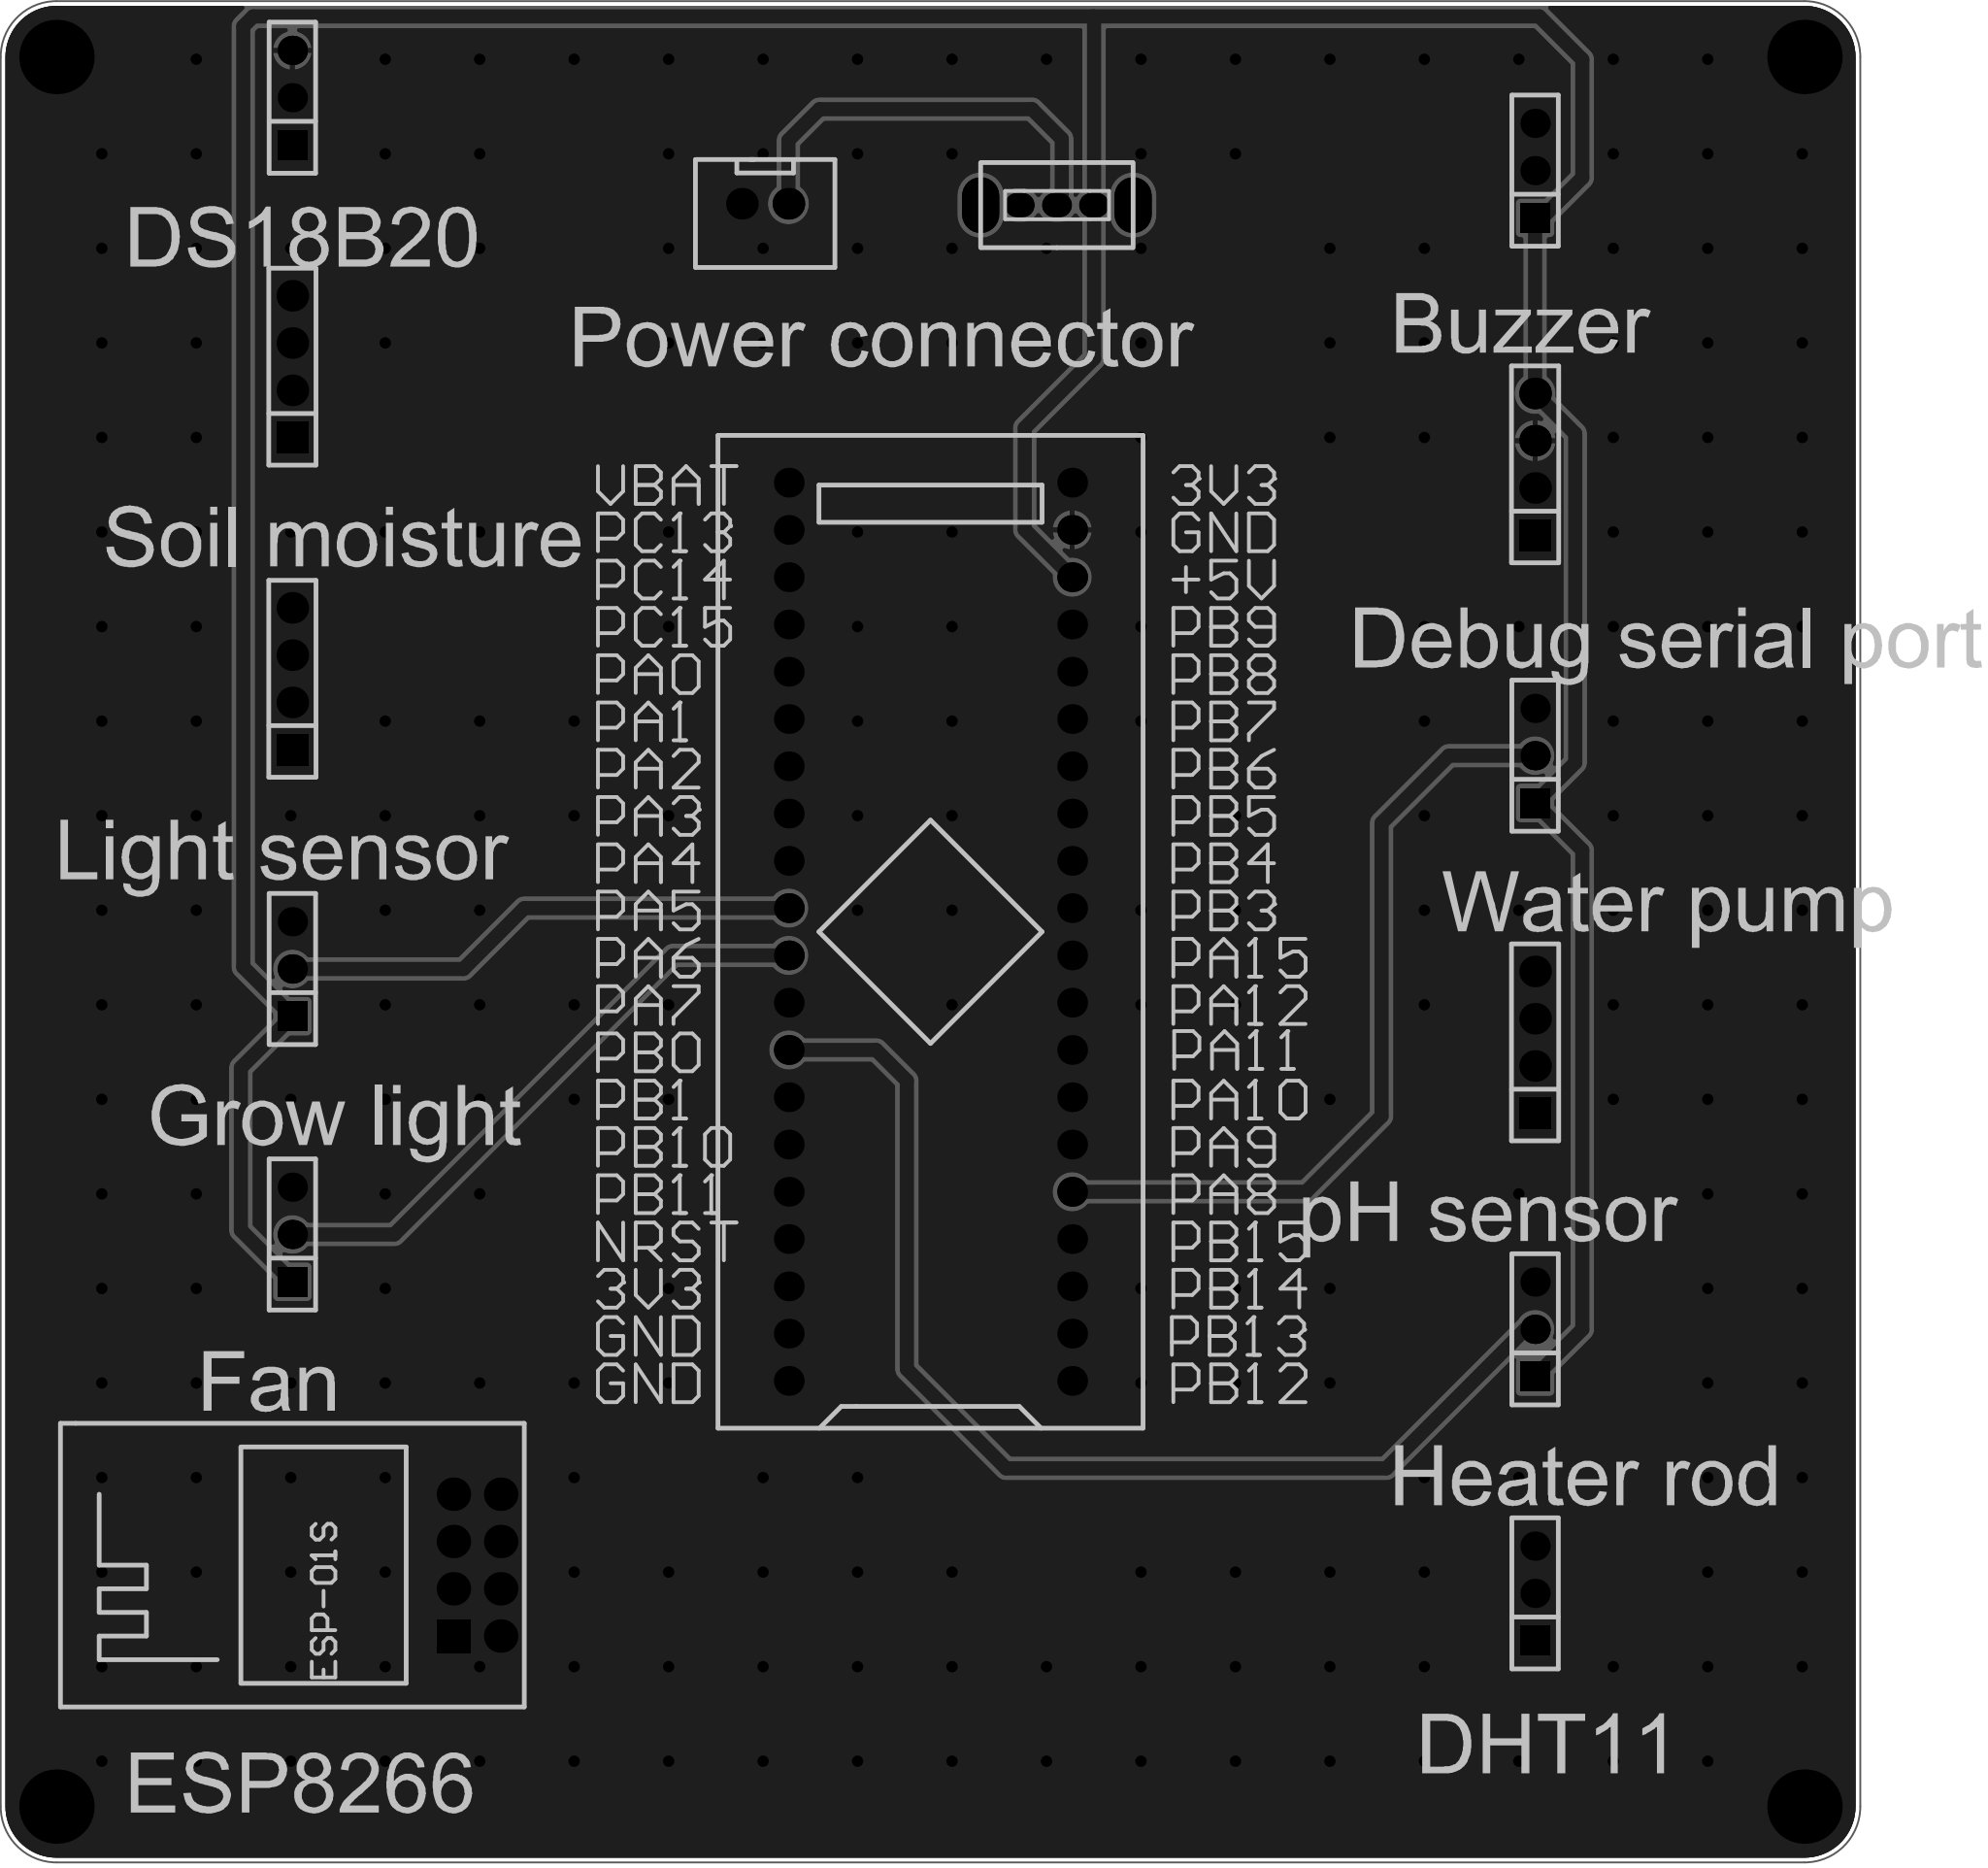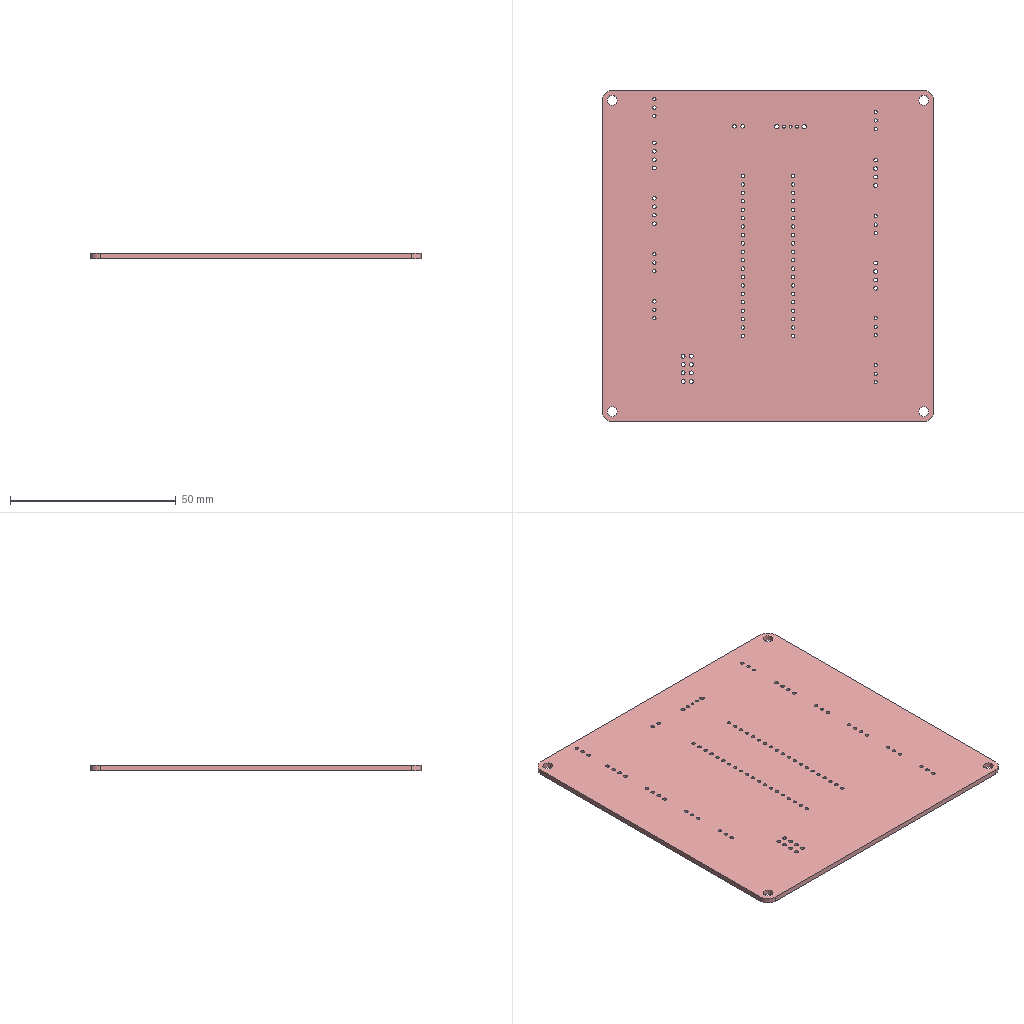Circuit board layout | Altium Designer | box 100 x 100 x 1.6 mm
Layer stack:
# Altium Designer layer stack of  (unit mm; dielectric type: 0 none, 1 core, 2 prepreg, 3 surface material)
index,name,kind,layer,copper_thickness_mm,dielectric_type,dielectric_thickness_mm,dielectric_material,dielectric_constant
0,Top Paste Mask Layer,other,,,,,,
1,Top Silkscreen Layer,other,,,,,,
2,Top Solder Mask Layer,dielectric,,,3,0.01,,3.3
3,Top Layer,copper,Top Layer,0.035,,,,
4,Dielectric1,dielectric,,,3,1.51,FR4,4.5
5,Bottom Layer,copper,Bottom Layer,0.035,,,,
6,Bottom Solder Mask Layer,dielectric,,,3,0.01,,3.3
7,Bottom Silkscreen Layer,other,,,,,,
8,Bottom Paste Mask Layer,other,,,,,,
# drill layer pairs: low layer,high layer
drill_pair,Top Layer,Bottom Layer
Part placement:
Designator,Comment,Layer,Footprint,Center-X(mm),Center-Y(mm),Rotation
U1,STM32F103C8T6-Card,TopLayer,CONN-TH_L53.3-W22.9_STM32F103C8T6-CARD,141.351,130.937,90
CN4,XH2.54*2P_straight,TopLayer,CONN-TH_2P-P2.50-XH2.54-2P,132.461,170.053,0
SW5,,TopLayer,拨动开关,148.148,169.978,180
H1,,TopLayer,HDR-TH_3P-P2.54-V-F,107.036,128.938,90
H2,,TopLayer,HDR-TH_4P-P2.54-V-F,173.863,156.05,90
H3,,TopLayer,HDR-TH_3P-P2.54-V-F,173.863,95.391,90
H4,,TopLayer,HDR-TH_4P-P2.54-V-F,107.036,161.298,90
H6,,TopLayer,HDR-TH_4P-P2.54-V-F,107.036,144.53,90
H7,,TopLayer,HDR-TH_4P-P2.54-V-F,173.863,124.996,90
H8,,TopLayer,HDR-TH_3P-P2.54-V-F,107.036,114.674,90
H9,,TopLayer,HDR-TH_3P-P2.54-V-F,173.863,140.398,90
H10,,TopLayer,HDR-TH_3P-P2.54-V-F,173.863,109.579,90
H11,,TopLayer,HDR-TH_3P-P2.54-V-F,107.036,175.749,90
H13,,TopLayer,HDR-TH_3P-P2.54-V-F,173.863,171.831,90
U2,ESP-01S,TopLayer,WIFIM-TH_ESP-01S,116.967,96.909,90
Pad and via stacks:
# Altium Designer via and pad stacks of  (unit mm). Each distinct definition once, with the count of objects using it.
# via: kind,start_layer,end_layer,hole_mm,diameter_mm,mode(0 simple;1 top-mid-bottom;2 full stack),diameter_per_layer,count,example_net
# pad: kind,layer,hole_mm,hole_type(0 round;1 square;2 slot),plating,top_size,top_shape(1 round;2 rect;3 octagon;9 rounded rect),mid_size,bottom_size,mode,footprint,size_per_layer,count,example
pad,Multi-Layer,3,0,plated,4x4,1,4x4,4x4,0,,,4,1
pad,Multi-Layer,1,0,plated,1.6x1.6,1,1.6x1.6,1.6x1.6,0,CONN-TH_L53.3-W22.9_STM32F103C8T6-CARD,,40,U1.1
pad,Multi-Layer,1.05,0,plated,1.7x1.7,1,1.7x1.7,1.7x1.7,0,CONN-TH_2P-P2.50-XH2.54-2P,,2,CN4.2
pad,Multi-Layer,0.8992,0,plated,1.6x1.3,1,1.6x1.3,1.6x1.3,0,\u00B2\u00A6\u00B6\u00AF\u00BF\u00AA\u00B9\u00D8,,3,SW5.1
pad,Multi-Layer,1.3,0,plated,3x1.999,1,3x1.999,3x1.999,0,\u00B2\u00A6\u00B6\u00AF\u00BF\u00AA\u00B9\u00D8,,2,SW5.4
pad,Multi-Layer,1.02,0,plated,1.575x1.575,1,1.575x1.575,1.575x1.575,0,HDR-TH_3P-P2.54-V-F,,14,H1.3
pad,Multi-Layer,1.02,0,plated,1.575x1.575,2,1.575x1.575,1.575x1.575,0,HDR-TH_3P-P2.54-V-F,,7,H1.1
pad,Multi-Layer,1.1,0,plated,1.7x1.7,2,1.7x1.7,1.7x1.7,0,HDR-TH_4P-P2.54-V-F,,4,H2.1
pad,Multi-Layer,1.1,0,plated,1.7x1.7,1,1.7x1.7,1.7x1.7,0,HDR-TH_4P-P2.54-V-F,,12,H2.2
pad,Multi-Layer,1.2,0,plated,1.8x1.8,2,1.8x1.8,1.8x1.8,0,WIFIM-TH_ESP-01S,,1,U2.1
pad,Multi-Layer,1.2,0,plated,1.8x1.8,1,1.8x1.8,1.8x1.8,0,WIFIM-TH_ESP-01S,,7,U2.2
via,Top Layer,Bottom Layer,0.3048,0.61,0,,243,GND
Copper pours:
name,layer,net,type(0 solid;1 hatched;2 none)
Bottom Layer-GND,Bottom Layer,GND,0
Bottom Layer-GND 1,Bottom Layer,GND,0
Top Layer-GND,Top Layer,GND,0
Top Layer-GND 1,Top Layer,GND,0
Design rules, without the lines most boards share:
# Altium Designer design rules of  (exported by Altium Designer, unit mm)
# columns: name | kind | enabled | priority | scope1 | scope2 | descriptor | typed fields (field=value)
Copper_copperRegion_copperThickness1oz | 0 | disabled | 4 | All | All | Clearance Constraint (Gap=5.984mil) (Disabled)(All),(All) | gap=0.152
Copper_copperRegion_copperThickness1oz_1 | 63 | disabled | 4 | All | All | Board Clearance Constraint (Gap=0mil) (Disabled)(All) |
Copper_copperRegion_Copper_copperRegion | 0 | disabled | 5 | All | All | Clearance Constraint (Gap=5.984mil) (Disabled)(All),(All) | gap=0.152
Copper_copperRegion_Copper_copperRegion_1 | 63 | disabled | 5 | All | All | Board Clearance Constraint (Gap=0mil) (Disabled)(All) |
copperThickness1oz | 0 | enabled | 6 | All | All | Clearance Constraint (Gap=5.984mil) (All),(All) | gap=0.152
copperThickness1oz_1 | 63 | enabled | 6 | All | All | Board Clearance Constraint (Gap=0mil) (All) |
copperRegion_copperThickness1oz | 20 | disabled | 1 | All | All | Polygon Connect Rule(Relief Connect )(Conductor Width=10mil) (Relief Angle=90 Angle) (Entries=4) (Air Gap Width=10mil) (Disabled)(All),(All) | connect_style(0=relief,1=direct,2=none)=0 relief_conductor_width=0.254 relief_entries=4
copperRegion_Copper_copperRegion | 20 | disabled | 2 | All | All | Polygon Connect Rule(Relief Connect )(Conductor Width=10mil) (Relief Angle=90 Angle) (Entries=4) (Air Gap Width=10mil) (Disabled)(All),(All) | connect_style(0=relief,1=direct,2=none)=0 relief_conductor_width=0.254 relief_entries=4
copperRegion | 20 | enabled | 3 | All | All | Polygon Connect Rule(Relief Connect )(Conductor Width=10mil) (Relief Angle=90 Angle) (Entries=4) (Air Gap Width=10mil) (All),(All) | connect_style(0=relief,1=direct,2=none)=0 relief_conductor_width=0.254 relief_entries=4